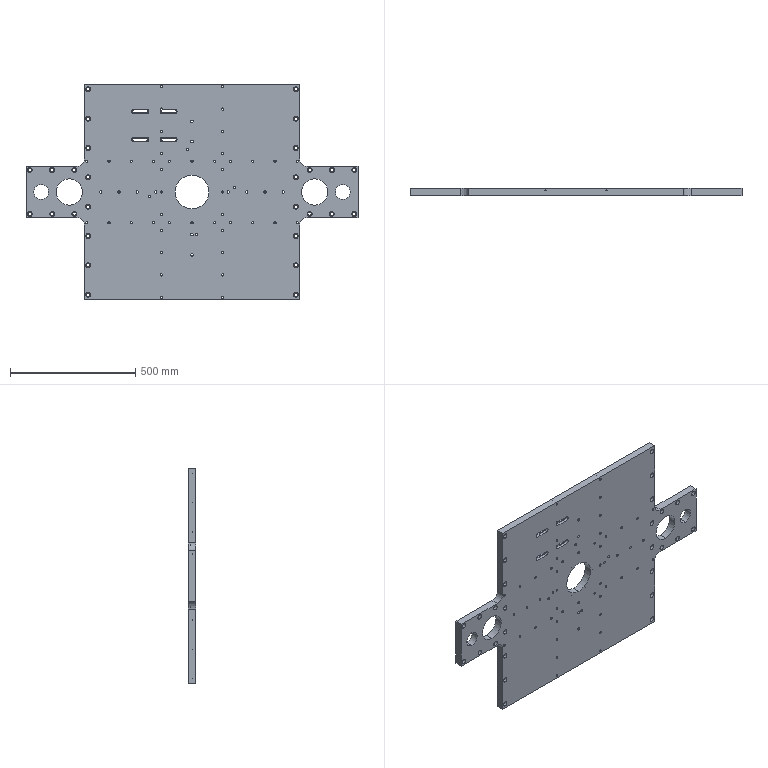Part | SolidWorks | features HoleWzd 7, MirrorPattern 4, Cut 3, DelFace 2, ICE 2, Cavity 1, CirPattern 1, Extrusion 1, Fillet 1, MoveFace 1 | 1 solid | 514 faces | box 1326 x 30 x 860 mm | volume 23495138 mm3 | cylinder 380 | plane 106 | cone 28 | commonest cylinder face diameters 9 x89 15 x88 13.5 x56 20 x56 10 x24 6.8 x16